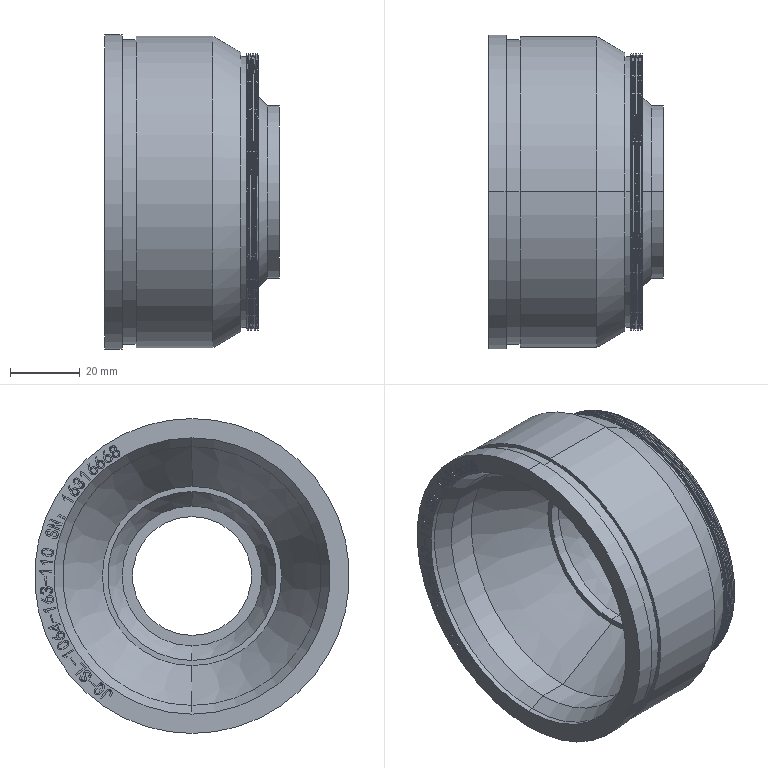Part | NX | features BREP 2 | 2 solids | 374 faces | box 50 x 90 x 90 mm | volume 105078 mm3 | plane 186 | spline 96 | cylinder 76 | cone 16 | commonest cylinder face diameters 84.3 x16 85 x13 79 x11 72 x4 34 x2 40 x2